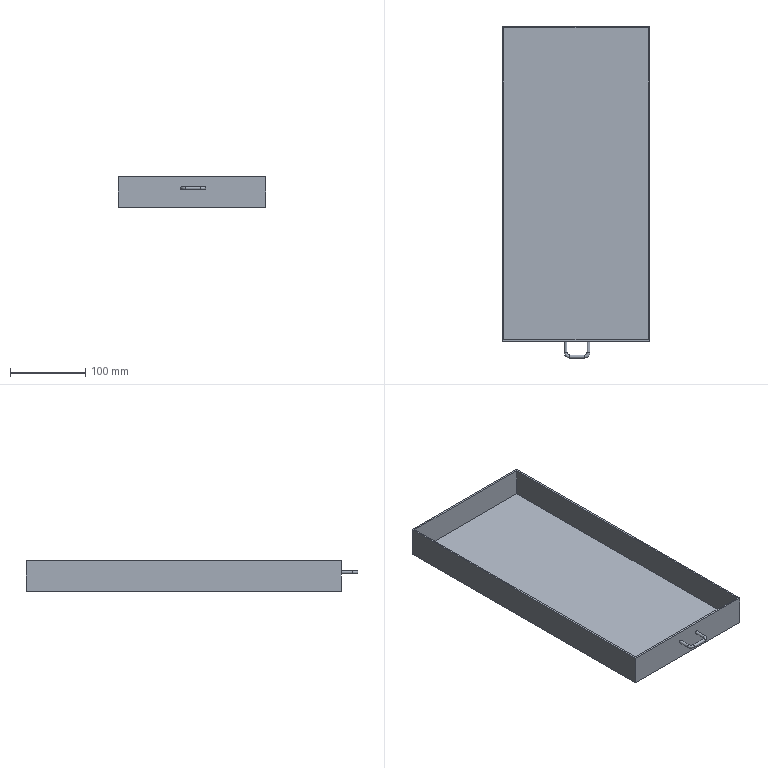Part | NX | features solid 2 | 1 solid | 16 faces | box 197 x 442 x 40 mm | volume 322426 mm3 | plane 11 | cylinder 3 | torus 2 | commonest cylinder face diameters 4 x3
STEP:
#1=CARTESIAN_POINT('',(-622.,-375.,-403.));
#2=VERTEX_POINT('',#1);
#3=CARTESIAN_POINT('',(-622.,-375.,-405.));
#4=DIRECTION('',(0.,-1.,0.));
#5=DIRECTION('',(0.,0.,1.));
#6=AXIS2_PLACEMENT_3D('',#3,#4,#5);
#7=CIRCLE('',#6,2.);
#8=EDGE_CURVE('',#2,#2,#7,.T.);
#9=ORIENTED_EDGE('',*,*,#8,.F.);
#10=EDGE_LOOP('',(#9));
#11=FACE_BOUND('',#10,.T.);
#12=CARTESIAN_POINT('',(-540.,-375.,-430.));
#13=VERTEX_POINT('',#12);
#14=CARTESIAN_POINT('',(-737.,-375.,-430.));
#15=VERTEX_POINT('',#14);
#16=CARTESIAN_POINT('',(-527.,-375.,-430.));
#17=DIRECTION('',(-1.,0.,0.));
#18=VECTOR('',#17,1000.);
#19=LINE('',#16,#18);
#20=EDGE_CURVE('',#13,#15,#19,.T.);
#21=ORIENTED_EDGE('',*,*,#20,.F.);
#22=CARTESIAN_POINT('',(-540.,-375.,-390.));
#23=VERTEX_POINT('',#22);
#24=CARTESIAN_POINT('',(-540.,-375.,-320.));
#25=DIRECTION('',(0.,0.,-1.));
#26=VECTOR('',#25,1000.);
#27=LINE('',#24,#26);
#28=EDGE_CURVE('',#23,#13,#27,.T.);
#29=ORIENTED_EDGE('',*,*,#28,.F.);
#30=CARTESIAN_POINT('',(-737.,-375.,-390.));
#31=VERTEX_POINT('',#30);
#32=CARTESIAN_POINT('',(-677.,-375.,-390.));
#33=DIRECTION('',(-1.,0.,0.));
#34=VECTOR('',#33,1000.);
#35=LINE('',#32,#34);
#36=EDGE_CURVE('',#23,#31,#35,.T.);
#37=ORIENTED_EDGE('',*,*,#36,.T.);
#38=CARTESIAN_POINT('',(-737.,-375.,-380.));
#39=DIRECTION('',(0.,0.,-1.));
#40=VECTOR('',#39,1000.);
#41=LINE('',#38,#40);
#42=EDGE_CURVE('',#31,#15,#41,.T.);
#43=ORIENTED_EDGE('',*,*,#42,.T.);
#44=EDGE_LOOP('',(#21,#29,#37,#43));
#45=FACE_BOUND('',#44,.T.);
#46=CARTESIAN_POINT('',(-652.,-375.,-403.));
#47=VERTEX_POINT('',#46);
#48=CARTESIAN_POINT('',(-652.,-375.,-405.));
#49=DIRECTION('',(0.,-1.,0.));
#50=DIRECTION('',(0.,0.,1.));
#51=AXIS2_PLACEMENT_3D('',#48,#49,#50);
#52=CIRCLE('',#51,2.);
#53=EDGE_CURVE('',#47,#47,#52,.T.);
#54=ORIENTED_EDGE('',*,*,#53,.F.);
#55=EDGE_LOOP('',(#54));
#56=FACE_BOUND('',#55,.T.);
#57=CARTESIAN_POINT('',(-527.,-375.,-380.));
#58=DIRECTION('',(0.,-1.,0.));
#59=DIRECTION('',(0.,0.,1.));
#60=AXIS2_PLACEMENT_3D('',#57,#58,#59);
#61=PLANE('',#60);
#62=ADVANCED_FACE('',(#11,#45,#56),#61,.T.);
#63=CARTESIAN_POINT('',(-734.5,-372.5,-427.5));
#64=VERTEX_POINT('',#63);
#65=CARTESIAN_POINT('',(-734.5,42.5,-427.5));
#66=VERTEX_POINT('',#65);
#67=CARTESIAN_POINT('',(-734.5,-252.5,-427.5));
#68=DIRECTION('',(0.,1.,0.));
#69=VECTOR('',#68,1000.);
#70=LINE('',#67,#69);
#71=EDGE_CURVE('',#64,#66,#70,.T.);
#72=ORIENTED_EDGE('',*,*,#71,.F.);
#73=CARTESIAN_POINT('',(-542.5,-372.5,-427.5));
#74=VERTEX_POINT('',#73);
#75=CARTESIAN_POINT('',(-677.,-372.5,-427.5));
#76=DIRECTION('',(-1.,0.,0.));
#77=VECTOR('',#76,1000.);
#78=LINE('',#75,#77);
#79=EDGE_CURVE('',#74,#64,#78,.T.);
#80=ORIENTED_EDGE('',*,*,#79,.F.);
#81=CARTESIAN_POINT('',(-542.5,42.5,-427.5));
#82=VERTEX_POINT('',#81);
#83=CARTESIAN_POINT('',(-542.5,-252.5,-427.5));
#84=DIRECTION('',(0.,-1.,0.));
#85=VECTOR('',#84,1000.);
#86=LINE('',#83,#85);
#87=EDGE_CURVE('',#82,#74,#86,.T.);
#88=ORIENTED_EDGE('',*,*,#87,.F.);
#89=CARTESIAN_POINT('',(-674.5,42.5,-427.5));
#90=DIRECTION('',(1.,0.,0.));
#91=VECTOR('',#90,1000.);
#92=LINE('',#89,#91);
#93=EDGE_CURVE('',#66,#82,#92,.T.);
#94=ORIENTED_EDGE('',*,*,#93,.F.);
#95=EDGE_LOOP('',(#72,#80,#88,#94));
#96=FACE_BOUND('',#95,.T.);
#97=CARTESIAN_POINT('',(-674.5,-252.5,-427.5));
#98=DIRECTION('',(0.,0.,-1.));
#99=DIRECTION('',(1.,0.,0.));
#100=AXIS2_PLACEMENT_3D('',#97,#98,#99);
#101=PLANE('',#100);
#102=ADVANCED_FACE('',(#96),#101,.F.);
#103=CARTESIAN_POINT('',(-737.,45.,-430.));
#104=VERTEX_POINT('',#103);
#105=CARTESIAN_POINT('',(-540.,45.,-430.));
#106=VERTEX_POINT('',#105);
#107=CARTESIAN_POINT('',(-674.5,45.,-430.));
#108=DIRECTION('',(1.,0.,0.));
#109=VECTOR('',#108,1000.);
#110=LINE('',#107,#109);
#111=EDGE_CURVE('',#104,#106,#110,.T.);
#112=ORIENTED_EDGE('',*,*,#111,.T.);
#113=CARTESIAN_POINT('',(-540.,-182.5,-430.));
#114=DIRECTION('',(0.,-1.,0.));
#115=VECTOR('',#114,1000.);
#116=LINE('',#113,#115);
#117=EDGE_CURVE('',#106,#13,#116,.T.);
#118=ORIENTED_EDGE('',*,*,#117,.T.);
#119=ORIENTED_EDGE('',*,*,#20,.T.);
#120=CARTESIAN_POINT('',(-737.,-182.5,-430.));
#121=DIRECTION('',(0.,1.,0.));
#122=VECTOR('',#121,1000.);
#123=LINE('',#120,#122);
#124=EDGE_CURVE('',#15,#104,#123,.T.);
#125=ORIENTED_EDGE('',*,*,#124,.T.);
#126=EDGE_LOOP('',(#112,#118,#119,#125));
#127=FACE_BOUND('',#126,.T.);
#128=CARTESIAN_POINT('',(-674.5,-182.5,-430.));
#129=DIRECTION('',(0.,0.,-1.));
#130=DIRECTION('',(1.,0.,0.));
#131=AXIS2_PLACEMENT_3D('',#128,#129,#130);
#132=PLANE('',#131);
#133=ADVANCED_FACE('',(#127),#132,.T.);
#134=CARTESIAN_POINT('',(-734.5,-372.5,-390.));
#135=VERTEX_POINT('',#134);
#136=CARTESIAN_POINT('',(-734.5,-372.5,-380.));
#137=DIRECTION('',(0.,0.,-1.));
#138=VECTOR('',#137,1000.);
#139=LINE('',#136,#138);
#140=EDGE_CURVE('',#135,#64,#139,.T.);
#141=ORIENTED_EDGE('',*,*,#140,.F.);
#142=CARTESIAN_POINT('',(-542.5,-372.5,-390.));
#143=VERTEX_POINT('',#142);
#144=CARTESIAN_POINT('',(-677.,-372.5,-390.));
#145=DIRECTION('',(1.,0.,0.));
#146=VECTOR('',#145,1000.);
#147=LINE('',#144,#146);
#148=EDGE_CURVE('',#135,#143,#147,.T.);
#149=ORIENTED_EDGE('',*,*,#148,.T.);
#150=CARTESIAN_POINT('',(-542.5,-372.5,-320.));
#151=DIRECTION('',(0.,0.,-1.));
#152=VECTOR('',#151,1000.);
#153=LINE('',#150,#152);
#154=EDGE_CURVE('',#143,#74,#153,.T.);
#155=ORIENTED_EDGE('',*,*,#154,.T.);
#156=ORIENTED_EDGE('',*,*,#79,.T.);
#157=EDGE_LOOP('',(#141,#149,#155,#156));
#158=FACE_BOUND('',#157,.T.);
#159=CARTESIAN_POINT('',(-677.,-372.5,-380.));
#160=DIRECTION('',(0.,1.,0.));
#161=DIRECTION('',(0.,0.,-1.));
#162=AXIS2_PLACEMENT_3D('',#159,#160,#161);
#163=PLANE('',#162);
#164=ADVANCED_FACE('',(#158),#163,.T.);
#165=ORIENTED_EDGE('',*,*,#124,.F.);
#166=ORIENTED_EDGE('',*,*,#42,.F.);
#167=CARTESIAN_POINT('',(-737.,45.,-390.));
#168=VERTEX_POINT('',#167);
#169=CARTESIAN_POINT('',(-737.,-372.5,-390.));
#170=DIRECTION('',(0.,1.,0.));
#171=VECTOR('',#170,1000.);
#172=LINE('',#169,#171);
#173=EDGE_CURVE('',#31,#168,#172,.T.);
#174=ORIENTED_EDGE('',*,*,#173,.T.);
#175=CARTESIAN_POINT('',(-737.,45.,-380.));
#176=DIRECTION('',(0.,0.,-1.));
#177=VECTOR('',#176,1000.);
#178=LINE('',#175,#177);
#179=EDGE_CURVE('',#168,#104,#178,.T.);
#180=ORIENTED_EDGE('',*,*,#179,.T.);
#181=EDGE_LOOP('',(#165,#166,#174,#180));
#182=FACE_BOUND('',#181,.T.);
#183=CARTESIAN_POINT('',(-737.,-375.,-380.));
#184=DIRECTION('',(-1.,0.,0.));
#185=DIRECTION('',(0.,0.,-1.));
#186=AXIS2_PLACEMENT_3D('',#183,#184,#185);
#187=PLANE('',#186);
#188=ADVANCED_FACE('',(#182),#187,.T.);
#189=ORIENTED_EDGE('',*,*,#117,.F.);
#190=CARTESIAN_POINT('',(-540.,45.,-390.));
#191=VERTEX_POINT('',#190);
#192=CARTESIAN_POINT('',(-540.,45.,-320.));
#193=DIRECTION('',(0.,0.,-1.));
#194=VECTOR('',#193,1000.);
#195=LINE('',#192,#194);
#196=EDGE_CURVE('',#191,#106,#195,.T.);
#197=ORIENTED_EDGE('',*,*,#196,.F.);
#198=CARTESIAN_POINT('',(-540.,80.624,-390.));
#199=DIRECTION('',(0.,-1.,0.));
#200=VECTOR('',#199,1000.);
#201=LINE('',#198,#200);
#202=EDGE_CURVE('',#191,#23,#201,.T.);
#203=ORIENTED_EDGE('',*,*,#202,.T.);
#204=ORIENTED_EDGE('',*,*,#28,.T.);
#205=EDGE_LOOP('',(#189,#197,#203,#204));
#206=FACE_BOUND('',#205,.T.);
#207=CARTESIAN_POINT('',(-540.,80.624,-320.));
#208=DIRECTION('',(-1.,0.,0.));
#209=DIRECTION('',(0.,0.,-1.));
#210=AXIS2_PLACEMENT_3D('',#207,#208,#209);
#211=PLANE('',#210);
#212=ADVANCED_FACE('',(#206),#211,.F.);
#213=ORIENTED_EDGE('',*,*,#148,.F.);
#214=CARTESIAN_POINT('',(-734.5,42.5,-390.));
#215=VERTEX_POINT('',#214);
#216=CARTESIAN_POINT('',(-734.5,-372.5,-390.));
#217=DIRECTION('',(0.,-1.,0.));
#218=VECTOR('',#217,1000.);
#219=LINE('',#216,#218);
#220=EDGE_CURVE('',#215,#135,#219,.T.);
#221=ORIENTED_EDGE('',*,*,#220,.F.);
#222=CARTESIAN_POINT('',(-542.5,42.5,-390.));
#223=VERTEX_POINT('',#222);
#224=CARTESIAN_POINT('',(-677.,42.5,-390.));
#225=DIRECTION('',(-1.,0.,0.));
#226=VECTOR('',#225,1000.);
#227=LINE('',#224,#226);
#228=EDGE_CURVE('',#223,#215,#227,.T.);
#229=ORIENTED_EDGE('',*,*,#228,.F.);
#230=CARTESIAN_POINT('',(-542.5,-372.5,-390.));
#231=DIRECTION('',(0.,1.,0.));
#232=VECTOR('',#231,1000.);
#233=LINE('',#230,#232);
#234=EDGE_CURVE('',#143,#223,#233,.T.);
#235=ORIENTED_EDGE('',*,*,#234,.F.);
#236=EDGE_LOOP('',(#213,#221,#229,#235));
#237=FACE_BOUND('',#236,.T.);
#238=ORIENTED_EDGE('',*,*,#173,.F.);
#239=ORIENTED_EDGE('',*,*,#36,.F.);
#240=ORIENTED_EDGE('',*,*,#202,.F.);
#241=CARTESIAN_POINT('',(-677.,45.,-390.));
#242=DIRECTION('',(1.,0.,0.));
#243=VECTOR('',#242,1000.);
#244=LINE('',#241,#243);
#245=EDGE_CURVE('',#168,#191,#244,.T.);
#246=ORIENTED_EDGE('',*,*,#245,.F.);
#247=EDGE_LOOP('',(#238,#239,#240,#246));
#248=FACE_BOUND('',#247,.T.);
#249=CARTESIAN_POINT('',(-677.,-372.5,-390.));
#250=DIRECTION('',(0.,0.,-1.));
#251=DIRECTION('',(1.,0.,0.));
#252=AXIS2_PLACEMENT_3D('',#249,#250,#251);
#253=PLANE('',#252);
#254=ADVANCED_FACE('',(#237,#248),#253,.F.);
#255=CARTESIAN_POINT('',(-734.5,42.5,-380.));
#256=DIRECTION('',(0.,0.,-1.));
#257=VECTOR('',#256,1000.);
#258=LINE('',#255,#257);
#259=EDGE_CURVE('',#215,#66,#258,.T.);
#260=ORIENTED_EDGE('',*,*,#259,.T.);
#261=ORIENTED_EDGE('',*,*,#93,.T.);
#262=CARTESIAN_POINT('',(-542.5,42.5,-320.));
#263=DIRECTION('',(0.,0.,-1.));
#264=VECTOR('',#263,1000.);
#265=LINE('',#262,#264);
#266=EDGE_CURVE('',#223,#82,#265,.T.);
#267=ORIENTED_EDGE('',*,*,#266,.F.);
#268=ORIENTED_EDGE('',*,*,#228,.T.);
#269=EDGE_LOOP('',(#260,#261,#267,#268));
#270=FACE_BOUND('',#269,.T.);
#271=CARTESIAN_POINT('',(-527.,42.5,-380.));
#272=DIRECTION('',(0.,-1.,0.));
#273=DIRECTION('',(0.,0.,1.));
#274=AXIS2_PLACEMENT_3D('',#271,#272,#273);
#275=PLANE('',#274);
#276=ADVANCED_FACE('',(#270),#275,.T.);
#277=ORIENTED_EDGE('',*,*,#111,.F.);
#278=ORIENTED_EDGE('',*,*,#179,.F.);
#279=ORIENTED_EDGE('',*,*,#245,.T.);
#280=ORIENTED_EDGE('',*,*,#196,.T.);
#281=EDGE_LOOP('',(#277,#278,#279,#280));
#282=FACE_BOUND('',#281,.T.);
#283=CARTESIAN_POINT('',(-677.,45.,-380.));
#284=DIRECTION('',(0.,1.,0.));
#285=DIRECTION('',(0.,0.,-1.));
#286=AXIS2_PLACEMENT_3D('',#283,#284,#285);
#287=PLANE('',#286);
#288=ADVANCED_FACE('',(#282),#287,.T.);
#289=ORIENTED_EDGE('',*,*,#87,.T.);
#290=ORIENTED_EDGE('',*,*,#154,.F.);
#291=ORIENTED_EDGE('',*,*,#234,.T.);
#292=ORIENTED_EDGE('',*,*,#266,.T.);
#293=EDGE_LOOP('',(#289,#290,#291,#292));
#294=FACE_BOUND('',#293,.T.);
#295=CARTESIAN_POINT('',(-542.5,10.624,-320.));
#296=DIRECTION('',(-1.,0.,0.));
#297=DIRECTION('',(0.,0.,-1.));
#298=AXIS2_PLACEMENT_3D('',#295,#296,#297);
#299=PLANE('',#298);
#300=ADVANCED_FACE('',(#294),#299,.T.);
#301=ORIENTED_EDGE('',*,*,#71,.T.);
#302=ORIENTED_EDGE('',*,*,#259,.F.);
#303=ORIENTED_EDGE('',*,*,#220,.T.);
#304=ORIENTED_EDGE('',*,*,#140,.T.);
#305=EDGE_LOOP('',(#301,#302,#303,#304));
#306=FACE_BOUND('',#305,.T.);
#307=CARTESIAN_POINT('',(-734.5,-252.5,-380.));
#308=DIRECTION('',(1.,0.,0.));
#309=DIRECTION('',(0.,0.,1.));
#310=AXIS2_PLACEMENT_3D('',#307,#308,#309);
#311=PLANE('',#310);
#312=ADVANCED_FACE('',(#306),#311,.T.);
#313=CARTESIAN_POINT('',(-622.,-390.,-403.));
#314=VERTEX_POINT('',#313);
#315=CARTESIAN_POINT('',(-622.,-390.,-405.));
#316=DIRECTION('',(0.,1.,0.));
#317=DIRECTION('',(0.,0.,1.));
#318=AXIS2_PLACEMENT_3D('',#315,#316,#317);
#319=CIRCLE('',#318,2.);
#320=EDGE_CURVE('',#314,#314,#319,.T.);
#321=ORIENTED_EDGE('',*,*,#320,.T.);
#322=EDGE_LOOP('',(#321));
#323=FACE_BOUND('',#322,.T.);
#324=ORIENTED_EDGE('',*,*,#8,.T.);
#325=EDGE_LOOP('',(#324));
#326=FACE_BOUND('',#325,.T.);
#327=CARTESIAN_POINT('',(-622.,-390.,-405.));
#328=DIRECTION('',(0.,1.,0.));
#329=DIRECTION('',(0.,0.,-1.));
#330=AXIS2_PLACEMENT_3D('',#327,#328,#329);
#331=CYLINDRICAL_SURFACE('',#330,2.);
#332=ADVANCED_FACE('',(#323,#326),#331,.T.);
#333=CARTESIAN_POINT('',(-627.,-395.,-403.));
#334=VERTEX_POINT('',#333);
#335=CARTESIAN_POINT('',(-627.,-395.,-405.));
#336=DIRECTION('',(1.,0.,0.));
#337=DIRECTION('',(0.,0.,1.));
#338=AXIS2_PLACEMENT_3D('',#335,#336,#337);
#339=CIRCLE('',#338,2.);
#340=EDGE_CURVE('',#334,#334,#339,.T.);
#341=ORIENTED_EDGE('',*,*,#340,.T.);
#342=EDGE_LOOP('',(#341));
#343=FACE_BOUND('',#342,.T.);
#344=ORIENTED_EDGE('',*,*,#320,.F.);
#345=EDGE_LOOP('',(#344));
#346=FACE_BOUND('',#345,.T.);
#347=CARTESIAN_POINT('',(-627.,-390.,-405.));
#348=DIRECTION('',(0.,0.,1.));
#349=DIRECTION('',(-1.,0.,0.));
#350=AXIS2_PLACEMENT_3D('',#347,#348,#349);
#351=TOROIDAL_SURFACE('',#350,5.,2.);
#352=ADVANCED_FACE('',(#343,#346),#351,.T.);
#353=CARTESIAN_POINT('',(-647.,-395.,-403.));
#354=VERTEX_POINT('',#353);
#355=CARTESIAN_POINT('',(-647.,-395.,-405.));
#356=DIRECTION('',(1.,0.,0.));
#357=DIRECTION('',(0.,0.,1.));
#358=AXIS2_PLACEMENT_3D('',#355,#356,#357);
#359=CIRCLE('',#358,2.);
#360=EDGE_CURVE('',#354,#354,#359,.T.);
#361=ORIENTED_EDGE('',*,*,#360,.T.);
#362=EDGE_LOOP('',(#361));
#363=FACE_BOUND('',#362,.T.);
#364=ORIENTED_EDGE('',*,*,#340,.F.);
#365=EDGE_LOOP('',(#364));
#366=FACE_BOUND('',#365,.T.);
#367=CARTESIAN_POINT('',(-647.,-395.,-405.));
#368=DIRECTION('',(1.,0.,0.));
#369=DIRECTION('',(0.,0.,1.));
#370=AXIS2_PLACEMENT_3D('',#367,#368,#369);
#371=CYLINDRICAL_SURFACE('',#370,2.);
#372=ADVANCED_FACE('',(#363,#366),#371,.T.);
#373=CARTESIAN_POINT('',(-652.,-390.,-403.));
#374=VERTEX_POINT('',#373);
#375=CARTESIAN_POINT('',(-652.,-390.,-405.));
#376=DIRECTION('',(0.,-1.,0.));
#377=DIRECTION('',(0.,0.,1.));
#378=AXIS2_PLACEMENT_3D('',#375,#376,#377);
#379=CIRCLE('',#378,2.);
#380=EDGE_CURVE('',#374,#374,#379,.T.);
#381=ORIENTED_EDGE('',*,*,#380,.T.);
#382=EDGE_LOOP('',(#381));
#383=FACE_BOUND('',#382,.T.);
#384=ORIENTED_EDGE('',*,*,#360,.F.);
#385=EDGE_LOOP('',(#384));
#386=FACE_BOUND('',#385,.T.);
#387=CARTESIAN_POINT('',(-647.,-390.,-405.));
#388=DIRECTION('',(0.,0.,1.));
#389=DIRECTION('',(-1.,0.,0.));
#390=AXIS2_PLACEMENT_3D('',#387,#388,#389);
#391=TOROIDAL_SURFACE('',#390,5.,2.);
#392=ADVANCED_FACE('',(#383,#386),#391,.T.);
#393=ORIENTED_EDGE('',*,*,#380,.F.);
#394=EDGE_LOOP('',(#393));
#395=FACE_BOUND('',#394,.T.);
#396=ORIENTED_EDGE('',*,*,#53,.T.);
#397=EDGE_LOOP('',(#396));
#398=FACE_BOUND('',#397,.T.);
#399=CARTESIAN_POINT('',(-652.,-390.,-405.));
#400=DIRECTION('',(0.,1.,0.));
#401=DIRECTION('',(0.,0.,-1.));
#402=AXIS2_PLACEMENT_3D('',#399,#400,#401);
#403=CYLINDRICAL_SURFACE('',#402,2.);
#404=ADVANCED_FACE('',(#395,#398),#403,.T.);
#405=CLOSED_SHELL('',(#62,#102,#133,#164,#188,#212,#254,#276,#288,#300,#312,#332,#352,#372,#392,#404));
#406=MANIFOLD_SOLID_BREP('',#405);
#407=(LENGTH_UNIT()NAMED_UNIT(*)SI_UNIT(.MILLI.,.METRE.));
#408=UNCERTAINTY_MEASURE_WITH_UNIT(LENGTH_MEASURE(0.00001),#407,'','');
#409=(NAMED_UNIT(*)PLANE_ANGLE_UNIT()SI_UNIT($,.RADIAN.));
#410=(NAMED_UNIT(*)SI_UNIT($,.STERADIAN.)SOLID_ANGLE_UNIT());
#411=(GEOMETRIC_REPRESENTATION_CONTEXT(3)GLOBAL_UNCERTAINTY_ASSIGNED_CONTEXT((#408))GLOBAL_UNIT_ASSIGNED_CONTEXT((#407,#409,#410))REPRESENTATION_CONTEXT('',''));
#412=ADVANCED_BREP_SHAPE_REPRESENTATION('',(#406),#411);